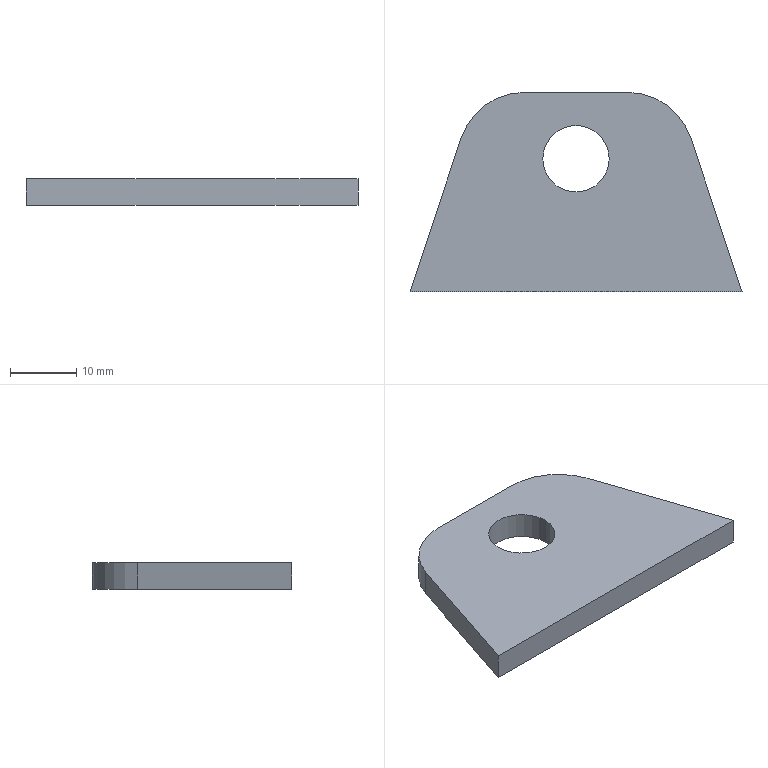Part | SolidWorks | features Extrusion 1 | 1 solid | 10 faces | box 50 x 30 x 4 mm | volume 4409 mm3 | plane 6 | cylinder 4 | commonest cylinder face diameters 10 x2 20 x2
STEP:
#1=CARTESIAN_POINT('',(20.,20.,4.));
#2=VERTEX_POINT('',#1);
#3=CARTESIAN_POINT('',(30.,20.,4.));
#4=VERTEX_POINT('',#3);
#5=CARTESIAN_POINT('',(25.,20.,4.));
#6=DIRECTION('',(0.,0.,1.));
#7=DIRECTION('',(1.,0.,0.));
#8=AXIS2_PLACEMENT_3D('',#5,#6,#7);
#9=CIRCLE('',#8,5.);
#10=EDGE_CURVE('',#2,#4,#9,.T.);
#11=ORIENTED_EDGE('',*,*,#10,.T.);
#12=CARTESIAN_POINT('',(30.,20.,0.));
#13=VERTEX_POINT('',#12);
#14=CARTESIAN_POINT('',(30.,20.,4.));
#15=DIRECTION('',(0.,0.,-1.));
#16=VECTOR('',#15,1000.);
#17=LINE('',#14,#16);
#18=EDGE_CURVE('',#4,#13,#17,.T.);
#19=ORIENTED_EDGE('',*,*,#18,.T.);
#20=CARTESIAN_POINT('',(20.,20.,0.));
#21=VERTEX_POINT('',#20);
#22=CARTESIAN_POINT('',(25.,20.,0.));
#23=DIRECTION('',(0.,0.,1.));
#24=DIRECTION('',(1.,0.,0.));
#25=AXIS2_PLACEMENT_3D('',#22,#23,#24);
#26=CIRCLE('',#25,5.);
#27=EDGE_CURVE('',#21,#13,#26,.T.);
#28=ORIENTED_EDGE('',*,*,#27,.F.);
#29=CARTESIAN_POINT('',(20.,20.,4.));
#30=DIRECTION('',(0.,0.,-1.));
#31=VECTOR('',#30,1000.);
#32=LINE('',#29,#31);
#33=EDGE_CURVE('',#2,#21,#32,.T.);
#34=ORIENTED_EDGE('',*,*,#33,.F.);
#35=EDGE_LOOP('',(#11,#19,#28,#34));
#36=FACE_OUTER_BOUND('',#35,.T.);
#37=CARTESIAN_POINT('',(25.,20.,4.));
#38=DIRECTION('',(0.,0.,-1.));
#39=DIRECTION('',(-1.,0.,0.));
#40=AXIS2_PLACEMENT_3D('',#37,#38,#39);
#41=CYLINDRICAL_SURFACE('',#40,5.);
#42=ADVANCED_FACE('',(#36),#41,.F.);
#43=CARTESIAN_POINT('',(7.721,23.162,4.));
#44=VERTEX_POINT('',#43);
#45=CARTESIAN_POINT('',(0.,0.,4.));
#46=VERTEX_POINT('',#45);
#47=CARTESIAN_POINT('',(7.721,23.162,4.));
#48=DIRECTION('',(-0.3162,-0.9487,0.));
#49=VECTOR('',#48,1000.);
#50=LINE('',#47,#49);
#51=EDGE_CURVE('',#44,#46,#50,.T.);
#52=ORIENTED_EDGE('',*,*,#51,.T.);
#53=CARTESIAN_POINT('',(50.,0.,4.));
#54=VERTEX_POINT('',#53);
#55=CARTESIAN_POINT('',(0.,0.,4.));
#56=DIRECTION('',(1.,0.,0.));
#57=VECTOR('',#56,1000.);
#58=LINE('',#55,#57);
#59=EDGE_CURVE('',#46,#54,#58,.T.);
#60=ORIENTED_EDGE('',*,*,#59,.T.);
#61=CARTESIAN_POINT('',(42.279,23.162,4.));
#62=VERTEX_POINT('',#61);
#63=CARTESIAN_POINT('',(50.,0.,4.));
#64=DIRECTION('',(-0.3162,0.9487,0.));
#65=VECTOR('',#64,1000.);
#66=LINE('',#63,#65);
#67=EDGE_CURVE('',#54,#62,#66,.T.);
#68=ORIENTED_EDGE('',*,*,#67,.T.);
#69=CARTESIAN_POINT('',(32.792,30.,4.));
#70=VERTEX_POINT('',#69);
#71=CARTESIAN_POINT('',(32.792,20.,4.));
#72=DIRECTION('',(0.,0.,1.));
#73=DIRECTION('',(1.,0.,0.));
#74=AXIS2_PLACEMENT_3D('',#71,#72,#73);
#75=CIRCLE('',#74,10.);
#76=EDGE_CURVE('',#62,#70,#75,.T.);
#77=ORIENTED_EDGE('',*,*,#76,.T.);
#78=CARTESIAN_POINT('',(17.208,30.,4.));
#79=VERTEX_POINT('',#78);
#80=CARTESIAN_POINT('',(32.792,30.,4.));
#81=DIRECTION('',(-1.,0.,0.));
#82=VECTOR('',#81,1000.);
#83=LINE('',#80,#82);
#84=EDGE_CURVE('',#70,#79,#83,.T.);
#85=ORIENTED_EDGE('',*,*,#84,.T.);
#86=CARTESIAN_POINT('',(17.208,20.,4.));
#87=DIRECTION('',(0.,0.,1.));
#88=DIRECTION('',(1.,0.,0.));
#89=AXIS2_PLACEMENT_3D('',#86,#87,#88);
#90=CIRCLE('',#89,10.);
#91=EDGE_CURVE('',#79,#44,#90,.T.);
#92=ORIENTED_EDGE('',*,*,#91,.T.);
#93=EDGE_LOOP('',(#52,#60,#68,#77,#85,#92));
#94=FACE_OUTER_BOUND('',#93,.T.);
#95=ORIENTED_EDGE('',*,*,#10,.F.);
#96=CARTESIAN_POINT('',(25.,20.,4.));
#97=DIRECTION('',(0.,0.,1.));
#98=DIRECTION('',(1.,0.,0.));
#99=AXIS2_PLACEMENT_3D('',#96,#97,#98);
#100=CIRCLE('',#99,5.);
#101=EDGE_CURVE('',#4,#2,#100,.T.);
#102=ORIENTED_EDGE('',*,*,#101,.F.);
#103=EDGE_LOOP('',(#95,#102));
#104=FACE_BOUND('',#103,.T.);
#105=CARTESIAN_POINT('',(32.792,20.,4.));
#106=DIRECTION('',(0.,0.,1.));
#107=DIRECTION('',(1.,0.,0.));
#108=AXIS2_PLACEMENT_3D('',#105,#106,#107);
#109=PLANE('',#108);
#110=ADVANCED_FACE('',(#94,#104),#109,.T.);
#111=CARTESIAN_POINT('',(7.721,23.162,0.));
#112=VERTEX_POINT('',#111);
#113=CARTESIAN_POINT('',(0.,0.,0.));
#114=VERTEX_POINT('',#113);
#115=CARTESIAN_POINT('',(7.721,23.162,0.));
#116=DIRECTION('',(-0.3162,-0.9487,0.));
#117=VECTOR('',#116,1000.);
#118=LINE('',#115,#117);
#119=EDGE_CURVE('',#112,#114,#118,.T.);
#120=ORIENTED_EDGE('',*,*,#119,.F.);
#121=CARTESIAN_POINT('',(17.208,30.,0.));
#122=VERTEX_POINT('',#121);
#123=CARTESIAN_POINT('',(17.208,20.,0.));
#124=DIRECTION('',(0.,0.,1.));
#125=DIRECTION('',(1.,0.,0.));
#126=AXIS2_PLACEMENT_3D('',#123,#124,#125);
#127=CIRCLE('',#126,10.);
#128=EDGE_CURVE('',#122,#112,#127,.T.);
#129=ORIENTED_EDGE('',*,*,#128,.F.);
#130=CARTESIAN_POINT('',(32.792,30.,0.));
#131=VERTEX_POINT('',#130);
#132=CARTESIAN_POINT('',(32.792,30.,0.));
#133=DIRECTION('',(-1.,0.,0.));
#134=VECTOR('',#133,1000.);
#135=LINE('',#132,#134);
#136=EDGE_CURVE('',#131,#122,#135,.T.);
#137=ORIENTED_EDGE('',*,*,#136,.F.);
#138=CARTESIAN_POINT('',(42.279,23.162,0.));
#139=VERTEX_POINT('',#138);
#140=CARTESIAN_POINT('',(32.792,20.,0.));
#141=DIRECTION('',(0.,0.,1.));
#142=DIRECTION('',(1.,0.,0.));
#143=AXIS2_PLACEMENT_3D('',#140,#141,#142);
#144=CIRCLE('',#143,10.);
#145=EDGE_CURVE('',#139,#131,#144,.T.);
#146=ORIENTED_EDGE('',*,*,#145,.F.);
#147=CARTESIAN_POINT('',(50.,0.,0.));
#148=VERTEX_POINT('',#147);
#149=CARTESIAN_POINT('',(50.,0.,0.));
#150=DIRECTION('',(-0.3162,0.9487,0.));
#151=VECTOR('',#150,1000.);
#152=LINE('',#149,#151);
#153=EDGE_CURVE('',#148,#139,#152,.T.);
#154=ORIENTED_EDGE('',*,*,#153,.F.);
#155=CARTESIAN_POINT('',(0.,0.,0.));
#156=DIRECTION('',(1.,0.,0.));
#157=VECTOR('',#156,1000.);
#158=LINE('',#155,#157);
#159=EDGE_CURVE('',#114,#148,#158,.T.);
#160=ORIENTED_EDGE('',*,*,#159,.F.);
#161=EDGE_LOOP('',(#120,#129,#137,#146,#154,#160));
#162=FACE_OUTER_BOUND('',#161,.T.);
#163=ORIENTED_EDGE('',*,*,#27,.T.);
#164=CARTESIAN_POINT('',(25.,20.,0.));
#165=DIRECTION('',(0.,0.,1.));
#166=DIRECTION('',(1.,0.,0.));
#167=AXIS2_PLACEMENT_3D('',#164,#165,#166);
#168=CIRCLE('',#167,5.);
#169=EDGE_CURVE('',#13,#21,#168,.T.);
#170=ORIENTED_EDGE('',*,*,#169,.T.);
#171=EDGE_LOOP('',(#163,#170));
#172=FACE_BOUND('',#171,.T.);
#173=CARTESIAN_POINT('',(32.792,20.,0.));
#174=DIRECTION('',(0.,0.,1.));
#175=DIRECTION('',(1.,0.,0.));
#176=AXIS2_PLACEMENT_3D('',#173,#174,#175);
#177=PLANE('',#176);
#178=ADVANCED_FACE('',(#162,#172),#177,.F.);
#179=ORIENTED_EDGE('',*,*,#119,.T.);
#180=CARTESIAN_POINT('',(0.,0.,4.));
#181=DIRECTION('',(0.,0.,-1.));
#182=VECTOR('',#181,1000.);
#183=LINE('',#180,#182);
#184=EDGE_CURVE('',#46,#114,#183,.T.);
#185=ORIENTED_EDGE('',*,*,#184,.F.);
#186=ORIENTED_EDGE('',*,*,#51,.F.);
#187=CARTESIAN_POINT('',(7.721,23.162,4.));
#188=DIRECTION('',(0.,0.,-1.));
#189=VECTOR('',#188,1000.);
#190=LINE('',#187,#189);
#191=EDGE_CURVE('',#44,#112,#190,.T.);
#192=ORIENTED_EDGE('',*,*,#191,.T.);
#193=EDGE_LOOP('',(#179,#185,#186,#192));
#194=FACE_OUTER_BOUND('',#193,.T.);
#195=CARTESIAN_POINT('',(7.721,23.162,4.));
#196=DIRECTION('',(0.9487,-0.3162,0.));
#197=DIRECTION('',(0.3162,0.9487,0.));
#198=AXIS2_PLACEMENT_3D('',#195,#196,#197);
#199=PLANE('',#198);
#200=ADVANCED_FACE('',(#194),#199,.F.);
#201=ORIENTED_EDGE('',*,*,#159,.T.);
#202=CARTESIAN_POINT('',(50.,0.,4.));
#203=DIRECTION('',(0.,0.,-1.));
#204=VECTOR('',#203,1000.);
#205=LINE('',#202,#204);
#206=EDGE_CURVE('',#54,#148,#205,.T.);
#207=ORIENTED_EDGE('',*,*,#206,.F.);
#208=ORIENTED_EDGE('',*,*,#59,.F.);
#209=ORIENTED_EDGE('',*,*,#184,.T.);
#210=EDGE_LOOP('',(#201,#207,#208,#209));
#211=FACE_OUTER_BOUND('',#210,.T.);
#212=CARTESIAN_POINT('',(0.,0.,4.));
#213=DIRECTION('',(0.,1.,0.));
#214=DIRECTION('',(0.,0.,1.));
#215=AXIS2_PLACEMENT_3D('',#212,#213,#214);
#216=PLANE('',#215);
#217=ADVANCED_FACE('',(#211),#216,.F.);
#218=ORIENTED_EDGE('',*,*,#153,.T.);
#219=CARTESIAN_POINT('',(42.279,23.162,4.));
#220=DIRECTION('',(0.,0.,-1.));
#221=VECTOR('',#220,1000.);
#222=LINE('',#219,#221);
#223=EDGE_CURVE('',#62,#139,#222,.T.);
#224=ORIENTED_EDGE('',*,*,#223,.F.);
#225=ORIENTED_EDGE('',*,*,#67,.F.);
#226=ORIENTED_EDGE('',*,*,#206,.T.);
#227=EDGE_LOOP('',(#218,#224,#225,#226));
#228=FACE_OUTER_BOUND('',#227,.T.);
#229=CARTESIAN_POINT('',(50.,0.,4.));
#230=DIRECTION('',(-0.9487,-0.3162,0.));
#231=DIRECTION('',(0.3162,-0.9487,0.));
#232=AXIS2_PLACEMENT_3D('',#229,#230,#231);
#233=PLANE('',#232);
#234=ADVANCED_FACE('',(#228),#233,.F.);
#235=ORIENTED_EDGE('',*,*,#145,.T.);
#236=CARTESIAN_POINT('',(32.792,30.,4.));
#237=DIRECTION('',(0.,0.,-1.));
#238=VECTOR('',#237,1000.);
#239=LINE('',#236,#238);
#240=EDGE_CURVE('',#70,#131,#239,.T.);
#241=ORIENTED_EDGE('',*,*,#240,.F.);
#242=ORIENTED_EDGE('',*,*,#76,.F.);
#243=ORIENTED_EDGE('',*,*,#223,.T.);
#244=EDGE_LOOP('',(#235,#241,#242,#243));
#245=FACE_OUTER_BOUND('',#244,.T.);
#246=CARTESIAN_POINT('',(32.792,20.,4.));
#247=DIRECTION('',(0.,0.,-1.));
#248=DIRECTION('',(-1.,0.,0.));
#249=AXIS2_PLACEMENT_3D('',#246,#247,#248);
#250=CYLINDRICAL_SURFACE('',#249,10.);
#251=ADVANCED_FACE('',(#245),#250,.T.);
#252=ORIENTED_EDGE('',*,*,#136,.T.);
#253=CARTESIAN_POINT('',(17.208,30.,4.));
#254=DIRECTION('',(0.,0.,-1.));
#255=VECTOR('',#254,1000.);
#256=LINE('',#253,#255);
#257=EDGE_CURVE('',#79,#122,#256,.T.);
#258=ORIENTED_EDGE('',*,*,#257,.F.);
#259=ORIENTED_EDGE('',*,*,#84,.F.);
#260=ORIENTED_EDGE('',*,*,#240,.T.);
#261=EDGE_LOOP('',(#252,#258,#259,#260));
#262=FACE_OUTER_BOUND('',#261,.T.);
#263=CARTESIAN_POINT('',(32.792,30.,4.));
#264=DIRECTION('',(0.,-1.,0.));
#265=DIRECTION('',(0.,0.,-1.));
#266=AXIS2_PLACEMENT_3D('',#263,#264,#265);
#267=PLANE('',#266);
#268=ADVANCED_FACE('',(#262),#267,.F.);
#269=ORIENTED_EDGE('',*,*,#128,.T.);
#270=ORIENTED_EDGE('',*,*,#191,.F.);
#271=ORIENTED_EDGE('',*,*,#91,.F.);
#272=ORIENTED_EDGE('',*,*,#257,.T.);
#273=EDGE_LOOP('',(#269,#270,#271,#272));
#274=FACE_OUTER_BOUND('',#273,.T.);
#275=CARTESIAN_POINT('',(17.208,20.,4.));
#276=DIRECTION('',(0.,0.,-1.));
#277=DIRECTION('',(-1.,0.,0.));
#278=AXIS2_PLACEMENT_3D('',#275,#276,#277);
#279=CYLINDRICAL_SURFACE('',#278,10.);
#280=ADVANCED_FACE('',(#274),#279,.T.);
#281=ORIENTED_EDGE('',*,*,#18,.F.);
#282=ORIENTED_EDGE('',*,*,#101,.T.);
#283=ORIENTED_EDGE('',*,*,#33,.T.);
#284=ORIENTED_EDGE('',*,*,#169,.F.);
#285=EDGE_LOOP('',(#281,#282,#283,#284));
#286=FACE_OUTER_BOUND('',#285,.T.);
#287=CARTESIAN_POINT('',(25.,20.,4.));
#288=DIRECTION('',(0.,0.,-1.));
#289=DIRECTION('',(-1.,0.,0.));
#290=AXIS2_PLACEMENT_3D('',#287,#288,#289);
#291=CYLINDRICAL_SURFACE('',#290,5.);
#292=ADVANCED_FACE('',(#286),#291,.F.);
#293=CLOSED_SHELL('',(#42,#110,#178,#200,#217,#234,#251,#268,#280,#292));
#294=MANIFOLD_SOLID_BREP('',#293);
#295=CARTESIAN_POINT('',(0.,0.,0.));
#296=DIRECTION('',(0.,0.,1.));
#297=DIRECTION('',(1.,0.,0.));
#298=AXIS2_PLACEMENT_3D('',#295,#296,#297);
#299=(LENGTH_UNIT()NAMED_UNIT(*)SI_UNIT(.MILLI.,.METRE.));
#300=UNCERTAINTY_MEASURE_WITH_UNIT(LENGTH_MEASURE(0.00001),#299,'','');
#301=(NAMED_UNIT(*)PLANE_ANGLE_UNIT()SI_UNIT($,.RADIAN.));
#302=(NAMED_UNIT(*)SI_UNIT($,.STERADIAN.)SOLID_ANGLE_UNIT());
#303=(GEOMETRIC_REPRESENTATION_CONTEXT(3)GLOBAL_UNCERTAINTY_ASSIGNED_CONTEXT((#300))GLOBAL_UNIT_ASSIGNED_CONTEXT((#299,#301,#302))REPRESENTATION_CONTEXT('',''));
#304=ADVANCED_BREP_SHAPE_REPRESENTATION('',(#294,#298),#303);